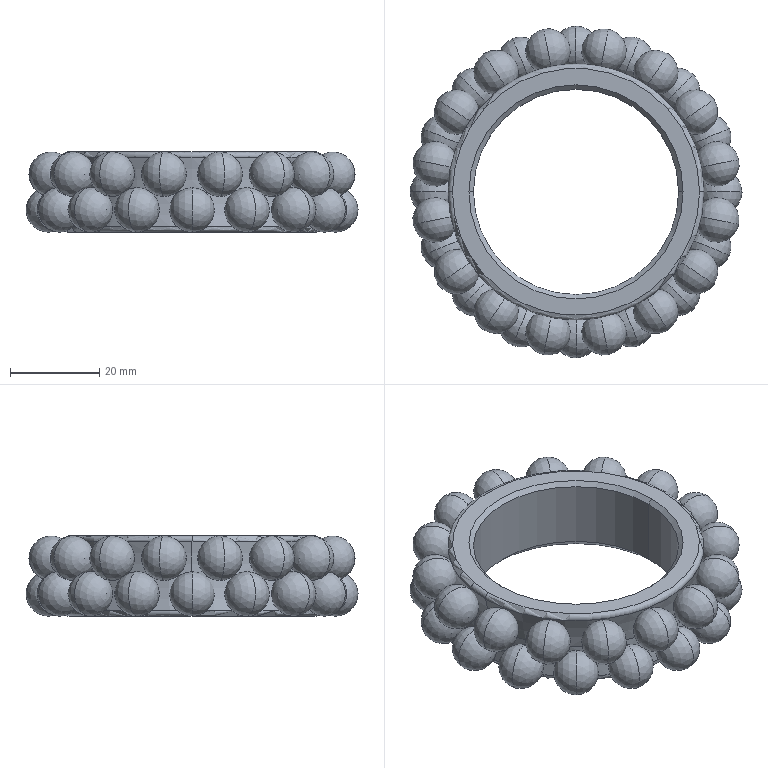Part | SolidWorks | features Chamfer 2, CirPattern 2, Revolution 2, Extrusion 1, Fillet 1, ICE 1, RevCut 1 | 33 solids | 80 faces | box 74.417 x 74.417 x 18 mm | volume 31009 mm3 | sphere 64 | torus 8 | cone 4 | cylinder 2 | plane 2 | commonest cylinder face diameters 46 x2